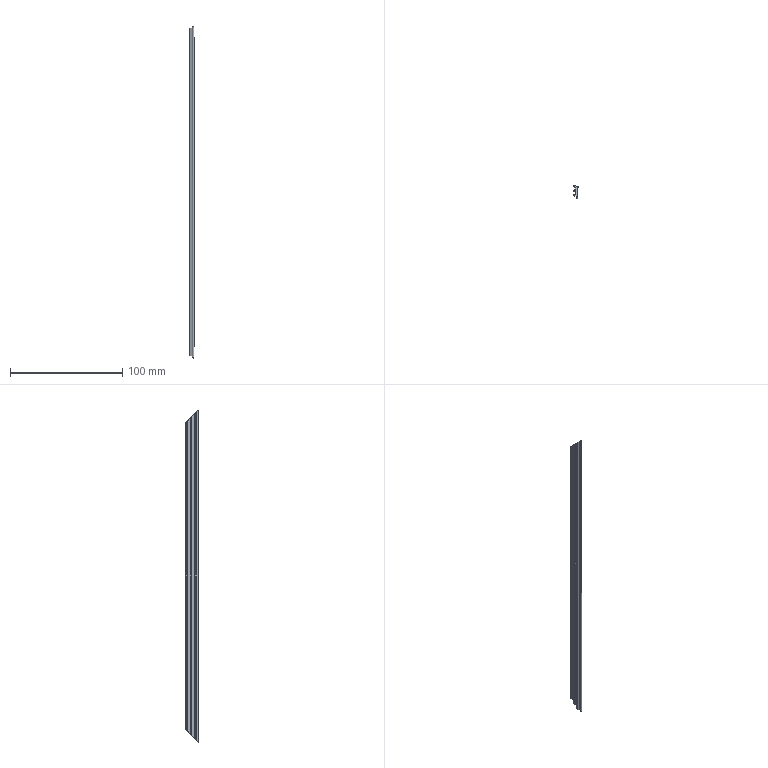Part | NX | features BREP 1 | 1 solid | 28 faces | box 3.587 x 11.224 x 296 mm | volume 6634 mm3 | plane 18 | cylinder 10 | commonest cylinder face diameters 0.4 x6 0.6 x2 1.942 x2
STEP:
#1=CARTESIAN_POINT('',(3.587,9.871,-138.128));
#2=VERTEX_POINT('',#1);
#3=CARTESIAN_POINT('',(3.287,9.567,-138.432));
#4=VERTEX_POINT('',#3);
#5=CARTESIAN_POINT('',(3.587,9.871,-138.128));
#6=CARTESIAN_POINT('',(3.589,9.693,-138.306));
#7=CARTESIAN_POINT('',(3.464,9.567,-138.432));
#8=CARTESIAN_POINT('',(3.287,9.567,-138.432));
#9=(BOUNDED_CURVE()B_SPLINE_CURVE(3,(#5,#6,#7,#8),.UNSPECIFIED.,.F.,.F.)B_SPLINE_CURVE_WITH_KNOTS((4,4),(4.699,6.283),.UNSPECIFIED.)CURVE()GEOMETRIC_REPRESENTATION_ITEM()RATIONAL_B_SPLINE_CURVE((1.,0.8015,0.8015,1.))REPRESENTATION_ITEM(''));
#10=EDGE_CURVE('',#2,#4,#9,.T.);
#11=ORIENTED_EDGE('',*,*,#10,.F.);
#12=CARTESIAN_POINT('',(3.587,9.871,138.128));
#13=VERTEX_POINT('',#12);
#14=CARTESIAN_POINT('',(3.587,9.871,148.));
#15=DIRECTION('',(0.,0.,-1.));
#16=VECTOR('',#15,1000.);
#17=LINE('',#14,#16);
#18=EDGE_CURVE('',#13,#2,#17,.T.);
#19=ORIENTED_EDGE('',*,*,#18,.F.);
#20=CARTESIAN_POINT('',(3.287,9.567,138.432));
#21=VERTEX_POINT('',#20);
#22=CARTESIAN_POINT('',(3.287,9.567,138.432));
#23=CARTESIAN_POINT('',(3.464,9.567,138.432));
#24=CARTESIAN_POINT('',(3.589,9.693,138.306));
#25=CARTESIAN_POINT('',(3.587,9.871,138.128));
#26=(BOUNDED_CURVE()B_SPLINE_CURVE(3,(#22,#23,#24,#25),.UNSPECIFIED.,.F.,.F.)B_SPLINE_CURVE_WITH_KNOTS((4,4),(3.142,4.726),.UNSPECIFIED.)CURVE()GEOMETRIC_REPRESENTATION_ITEM()RATIONAL_B_SPLINE_CURVE((1.,0.8015,0.8015,1.))REPRESENTATION_ITEM(''));
#27=EDGE_CURVE('',#21,#13,#26,.T.);
#28=ORIENTED_EDGE('',*,*,#27,.F.);
#29=CARTESIAN_POINT('',(3.287,9.567,148.));
#30=DIRECTION('',(0.,0.,-1.));
#31=VECTOR('',#30,1000.);
#32=LINE('',#29,#31);
#33=EDGE_CURVE('',#21,#4,#32,.T.);
#34=ORIENTED_EDGE('',*,*,#33,.T.);
#35=EDGE_LOOP('',(#11,#19,#28,#34));
#36=FACE_BOUND('',#35,.T.);
#37=CARTESIAN_POINT('',(3.287,9.867,148.));
#38=DIRECTION('',(0.,0.,-1.));
#39=DIRECTION('',(-1.,0.,0.));
#40=AXIS2_PLACEMENT_3D('',#37,#38,#39);
#41=CYLINDRICAL_SURFACE('',#40,0.3);
#42=ADVANCED_FACE('',(#36),#41,.T.);
#43=CARTESIAN_POINT('',(3.447,10.36,-137.639));
#44=VERTEX_POINT('',#43);
#45=CARTESIAN_POINT('',(3.447,10.36,-137.639));
#46=CARTESIAN_POINT('',(3.536,10.211,-137.788));
#47=CARTESIAN_POINT('',(3.584,10.044,-137.955));
#48=CARTESIAN_POINT('',(3.587,9.871,-138.128));
#49=(BOUNDED_CURVE()B_SPLINE_CURVE(3,(#45,#46,#47,#48),.UNSPECIFIED.,.F.,.F.)B_SPLINE_CURVE_WITH_KNOTS((4,4),(4.169,4.699),.UNSPECIFIED.)CURVE()GEOMETRIC_REPRESENTATION_ITEM()RATIONAL_B_SPLINE_CURVE((1.,0.9767,0.9767,1.))REPRESENTATION_ITEM(''));
#50=EDGE_CURVE('',#44,#2,#49,.T.);
#51=ORIENTED_EDGE('',*,*,#50,.F.);
#52=CARTESIAN_POINT('',(3.447,10.36,137.639));
#53=VERTEX_POINT('',#52);
#54=CARTESIAN_POINT('',(3.447,10.36,148.));
#55=DIRECTION('',(0.,0.,-1.));
#56=VECTOR('',#55,1000.);
#57=LINE('',#54,#56);
#58=EDGE_CURVE('',#53,#44,#57,.T.);
#59=ORIENTED_EDGE('',*,*,#58,.F.);
#60=CARTESIAN_POINT('',(3.587,9.871,138.128));
#61=CARTESIAN_POINT('',(3.584,10.044,137.955));
#62=CARTESIAN_POINT('',(3.536,10.211,137.788));
#63=CARTESIAN_POINT('',(3.447,10.36,137.639));
#64=(BOUNDED_CURVE()B_SPLINE_CURVE(3,(#60,#61,#62,#63),.UNSPECIFIED.,.F.,.F.)B_SPLINE_CURVE_WITH_KNOTS((4,4),(4.726,5.256),.UNSPECIFIED.)CURVE()GEOMETRIC_REPRESENTATION_ITEM()RATIONAL_B_SPLINE_CURVE((1.,0.9767,0.9767,1.))REPRESENTATION_ITEM(''));
#65=EDGE_CURVE('',#13,#53,#64,.T.);
#66=ORIENTED_EDGE('',*,*,#65,.F.);
#67=ORIENTED_EDGE('',*,*,#18,.T.);
#68=EDGE_LOOP('',(#51,#59,#66,#67));
#69=FACE_BOUND('',#68,.T.);
#70=CARTESIAN_POINT('',(2.616,9.857,148.));
#71=DIRECTION('',(0.,0.,-1.));
#72=DIRECTION('',(-1.,0.,0.));
#73=AXIS2_PLACEMENT_3D('',#70,#71,#72);
#74=CYLINDRICAL_SURFACE('',#73,0.971);
#75=ADVANCED_FACE('',(#69),#74,.T.);
#76=CARTESIAN_POINT('',(0.2517,11.216,-136.783));
#77=VERTEX_POINT('',#76);
#78=CARTESIAN_POINT('',(-63.462,28.281,-119.717));
#79=DIRECTION('',(0.9352,-0.2505,-0.2505));
#80=VECTOR('',#79,1000.);
#81=LINE('',#78,#80);
#82=EDGE_CURVE('',#77,#44,#81,.T.);
#83=ORIENTED_EDGE('',*,*,#82,.F.);
#84=CARTESIAN_POINT('',(0.2517,11.216,136.783));
#85=VERTEX_POINT('',#84);
#86=CARTESIAN_POINT('',(0.2517,11.216,148.));
#87=DIRECTION('',(0.,0.,-1.));
#88=VECTOR('',#87,1000.);
#89=LINE('',#86,#88);
#90=EDGE_CURVE('',#85,#77,#89,.T.);
#91=ORIENTED_EDGE('',*,*,#90,.F.);
#92=CARTESIAN_POINT('',(5.874,9.71,138.289));
#93=DIRECTION('',(-0.9352,0.2505,-0.2505));
#94=VECTOR('',#93,1000.);
#95=LINE('',#92,#94);
#96=EDGE_CURVE('',#53,#85,#95,.T.);
#97=ORIENTED_EDGE('',*,*,#96,.F.);
#98=ORIENTED_EDGE('',*,*,#58,.T.);
#99=EDGE_LOOP('',(#83,#91,#97,#98));
#100=FACE_BOUND('',#99,.T.);
#101=CARTESIAN_POINT('',(3.447,10.36,148.));
#102=DIRECTION('',(-0.2587,-0.9659,0.));
#103=DIRECTION('',(-0.9659,0.2587,0.));
#104=AXIS2_PLACEMENT_3D('',#101,#102,#103);
#105=PLANE('',#104);
#106=ADVANCED_FACE('',(#100),#105,.F.);
#107=CARTESIAN_POINT('',(0.,11.022,-136.976));
#108=VERTEX_POINT('',#107);
#109=CARTESIAN_POINT('',(0.,11.022,-136.976));
#110=CARTESIAN_POINT('',(0.,11.165,-136.833));
#111=CARTESIAN_POINT('',(0.1135,11.253,-136.746));
#112=CARTESIAN_POINT('',(0.2517,11.216,-136.783));
#113=(BOUNDED_CURVE()B_SPLINE_CURVE(3,(#109,#110,#111,#112),.UNSPECIFIED.,.F.,.F.)B_SPLINE_CURVE_WITH_KNOTS((4,4),(1.571,3.403),.UNSPECIFIED.)CURVE()GEOMETRIC_REPRESENTATION_ITEM()RATIONAL_B_SPLINE_CURVE((1.,0.7392,0.7392,1.))REPRESENTATION_ITEM(''));
#114=EDGE_CURVE('',#108,#77,#113,.T.);
#115=ORIENTED_EDGE('',*,*,#114,.F.);
#116=CARTESIAN_POINT('',(0.,11.022,136.976));
#117=VERTEX_POINT('',#116);
#118=CARTESIAN_POINT('',(0.,11.022,148.));
#119=DIRECTION('',(0.,0.,-1.));
#120=VECTOR('',#119,1000.);
#121=LINE('',#118,#120);
#122=EDGE_CURVE('',#117,#108,#121,.T.);
#123=ORIENTED_EDGE('',*,*,#122,.F.);
#124=CARTESIAN_POINT('',(0.2517,11.216,136.783));
#125=CARTESIAN_POINT('',(0.1135,11.253,136.746));
#126=CARTESIAN_POINT('',(0.,11.165,136.833));
#127=CARTESIAN_POINT('',(0.,11.022,136.976));
#128=(BOUNDED_CURVE()B_SPLINE_CURVE(3,(#124,#125,#126,#127),.UNSPECIFIED.,.F.,.F.)B_SPLINE_CURVE_WITH_KNOTS((4,4),(6.021,7.854),.UNSPECIFIED.)CURVE()GEOMETRIC_REPRESENTATION_ITEM()RATIONAL_B_SPLINE_CURVE((1.,0.7392,0.7392,1.))REPRESENTATION_ITEM(''));
#129=EDGE_CURVE('',#85,#117,#128,.T.);
#130=ORIENTED_EDGE('',*,*,#129,.F.);
#131=ORIENTED_EDGE('',*,*,#90,.T.);
#132=EDGE_LOOP('',(#115,#123,#130,#131));
#133=FACE_BOUND('',#132,.T.);
#134=CARTESIAN_POINT('',(0.2,11.022,148.));
#135=DIRECTION('',(0.,0.,-1.));
#136=DIRECTION('',(-1.,0.,0.));
#137=AXIS2_PLACEMENT_3D('',#134,#135,#136);
#138=CYLINDRICAL_SURFACE('',#137,0.2);
#139=ADVANCED_FACE('',(#133),#138,.T.);
#140=CARTESIAN_POINT('',(0.,10.432,-137.567));
#141=VERTEX_POINT('',#140);
#142=CARTESIAN_POINT('',(0.,153.511,5.512));
#143=DIRECTION('',(0.,0.7071,0.7071));
#144=VECTOR('',#143,1000.);
#145=LINE('',#142,#144);
#146=EDGE_CURVE('',#141,#108,#145,.T.);
#147=ORIENTED_EDGE('',*,*,#146,.F.);
#148=CARTESIAN_POINT('',(0.,10.432,137.567));
#149=VERTEX_POINT('',#148);
#150=CARTESIAN_POINT('',(0.,10.432,148.));
#151=DIRECTION('',(0.,0.,-1.));
#152=VECTOR('',#151,1000.);
#153=LINE('',#150,#152);
#154=EDGE_CURVE('',#149,#141,#153,.T.);
#155=ORIENTED_EDGE('',*,*,#154,.F.);
#156=CARTESIAN_POINT('',(0.,5.511,142.488));
#157=DIRECTION('',(0.,-0.7071,0.7071));
#158=VECTOR('',#157,1000.);
#159=LINE('',#156,#158);
#160=EDGE_CURVE('',#117,#149,#159,.T.);
#161=ORIENTED_EDGE('',*,*,#160,.F.);
#162=ORIENTED_EDGE('',*,*,#122,.T.);
#163=EDGE_LOOP('',(#147,#155,#161,#162));
#164=FACE_BOUND('',#163,.T.);
#165=CARTESIAN_POINT('',(0.,11.022,148.));
#166=DIRECTION('',(1.,0.,0.));
#167=DIRECTION('',(0.,1.,0.));
#168=AXIS2_PLACEMENT_3D('',#165,#166,#167);
#169=PLANE('',#168);
#170=ADVANCED_FACE('',(#164),#169,.F.);
#171=CARTESIAN_POINT('',(0.1483,10.238,-137.76));
#172=VERTEX_POINT('',#171);
#173=CARTESIAN_POINT('',(0.1483,10.238,-137.76));
#174=CARTESIAN_POINT('',(0.05733,10.263,-137.736));
#175=CARTESIAN_POINT('',(0.,10.338,-137.661));
#176=CARTESIAN_POINT('',(0.,10.432,-137.567));
#177=(BOUNDED_CURVE()B_SPLINE_CURVE(3,(#173,#174,#175,#176),.UNSPECIFIED.,.F.,.F.)B_SPLINE_CURVE_WITH_KNOTS((4,4),(0.2616,1.571),.UNSPECIFIED.)CURVE()GEOMETRIC_REPRESENTATION_ITEM()RATIONAL_B_SPLINE_CURVE((1.,0.8622,0.8622,1.))REPRESENTATION_ITEM(''));
#178=EDGE_CURVE('',#172,#141,#177,.T.);
#179=ORIENTED_EDGE('',*,*,#178,.F.);
#180=CARTESIAN_POINT('',(0.1483,10.238,137.76));
#181=VERTEX_POINT('',#180);
#182=CARTESIAN_POINT('',(0.1483,10.238,148.));
#183=DIRECTION('',(0.,0.,-1.));
#184=VECTOR('',#183,1000.);
#185=LINE('',#182,#184);
#186=EDGE_CURVE('',#181,#172,#185,.T.);
#187=ORIENTED_EDGE('',*,*,#186,.F.);
#188=CARTESIAN_POINT('',(0.,10.432,137.567));
#189=CARTESIAN_POINT('',(0.,10.338,137.661));
#190=CARTESIAN_POINT('',(0.05733,10.263,137.736));
#191=CARTESIAN_POINT('',(0.1483,10.238,137.76));
#192=(BOUNDED_CURVE()B_SPLINE_CURVE(3,(#188,#189,#190,#191),.UNSPECIFIED.,.F.,.F.)B_SPLINE_CURVE_WITH_KNOTS((4,4),(1.571,2.88),.UNSPECIFIED.)CURVE()GEOMETRIC_REPRESENTATION_ITEM()RATIONAL_B_SPLINE_CURVE((1.,0.8622,0.8622,1.))REPRESENTATION_ITEM(''));
#193=EDGE_CURVE('',#149,#181,#192,.T.);
#194=ORIENTED_EDGE('',*,*,#193,.F.);
#195=ORIENTED_EDGE('',*,*,#154,.T.);
#196=EDGE_LOOP('',(#179,#187,#194,#195));
#197=FACE_BOUND('',#196,.T.);
#198=CARTESIAN_POINT('',(0.2,10.432,148.));
#199=DIRECTION('',(0.,0.,-1.));
#200=DIRECTION('',(-1.,0.,0.));
#201=AXIS2_PLACEMENT_3D('',#198,#199,#200);
#202=CYLINDRICAL_SURFACE('',#201,0.2);
#203=ADVANCED_FACE('',(#197),#202,.T.);
#204=CARTESIAN_POINT('',(0.854,10.05,-137.949));
#205=VERTEX_POINT('',#204);
#206=CARTESIAN_POINT('',(-66.763,28.152,-119.847));
#207=DIRECTION('',(-0.9352,0.2504,0.2504));
#208=VECTOR('',#207,1000.);
#209=LINE('',#206,#208);
#210=EDGE_CURVE('',#205,#172,#209,.T.);
#211=ORIENTED_EDGE('',*,*,#210,.F.);
#212=CARTESIAN_POINT('',(0.854,10.05,137.949));
#213=VERTEX_POINT('',#212);
#214=CARTESIAN_POINT('',(0.854,10.05,148.));
#215=DIRECTION('',(0.,0.,-1.));
#216=VECTOR('',#215,1000.);
#217=LINE('',#214,#216);
#218=EDGE_CURVE('',#213,#205,#217,.T.);
#219=ORIENTED_EDGE('',*,*,#218,.F.);
#220=CARTESIAN_POINT('',(2.546,9.597,138.402));
#221=DIRECTION('',(0.9352,-0.2504,0.2504));
#222=VECTOR('',#221,1000.);
#223=LINE('',#220,#222);
#224=EDGE_CURVE('',#181,#213,#223,.T.);
#225=ORIENTED_EDGE('',*,*,#224,.F.);
#226=ORIENTED_EDGE('',*,*,#186,.T.);
#227=EDGE_LOOP('',(#211,#219,#225,#226));
#228=FACE_BOUND('',#227,.T.);
#229=CARTESIAN_POINT('',(0.1483,10.238,148.));
#230=DIRECTION('',(0.2586,0.966,0.));
#231=DIRECTION('',(0.,0.,-1.));
#232=AXIS2_PLACEMENT_3D('',#229,#230,#231);
#233=PLANE('',#232);
#234=ADVANCED_FACE('',(#228),#233,.F.);
#235=CARTESIAN_POINT('',(1.256,6.926,-141.073));
#236=VERTEX_POINT('',#235);
#237=CARTESIAN_POINT('',(-17.383,151.851,3.853));
#238=DIRECTION('',(-0.09057,0.7042,0.7042));
#239=VECTOR('',#238,1000.);
#240=LINE('',#237,#239);
#241=EDGE_CURVE('',#236,#205,#240,.T.);
#242=ORIENTED_EDGE('',*,*,#241,.F.);
#243=CARTESIAN_POINT('',(1.256,6.926,141.073));
#244=VERTEX_POINT('',#243);
#245=CARTESIAN_POINT('',(1.256,6.926,148.));
#246=DIRECTION('',(0.,0.,-1.));
#247=VECTOR('',#246,1000.);
#248=LINE('',#245,#247);
#249=EDGE_CURVE('',#244,#236,#248,.T.);
#250=ORIENTED_EDGE('',*,*,#249,.F.);
#251=CARTESIAN_POINT('',(1.495,5.065,142.933));
#252=DIRECTION('',(0.09057,-0.7042,0.7042));
#253=VECTOR('',#252,1000.);
#254=LINE('',#251,#253);
#255=EDGE_CURVE('',#213,#244,#254,.T.);
#256=ORIENTED_EDGE('',*,*,#255,.F.);
#257=ORIENTED_EDGE('',*,*,#218,.T.);
#258=EDGE_LOOP('',(#242,#250,#256,#257));
#259=FACE_BOUND('',#258,.T.);
#260=CARTESIAN_POINT('',(0.854,10.05,148.));
#261=DIRECTION('',(0.9918,0.1276,0.));
#262=DIRECTION('',(0.,0.,-1.));
#263=AXIS2_PLACEMENT_3D('',#260,#261,#262);
#264=PLANE('',#263);
#265=ADVANCED_FACE('',(#259),#264,.F.);
#266=CARTESIAN_POINT('',(0.2517,7.195,-140.804));
#267=VERTEX_POINT('',#266);
#268=CARTESIAN_POINT('',(-66.433,25.048,-122.951));
#269=DIRECTION('',(0.9352,-0.2504,-0.2504));
#270=VECTOR('',#269,1000.);
#271=LINE('',#268,#270);
#272=EDGE_CURVE('',#267,#236,#271,.T.);
#273=ORIENTED_EDGE('',*,*,#272,.F.);
#274=CARTESIAN_POINT('',(0.2517,7.195,140.804));
#275=VERTEX_POINT('',#274);
#276=CARTESIAN_POINT('',(0.2517,7.195,148.));
#277=DIRECTION('',(0.,0.,-1.));
#278=VECTOR('',#277,1000.);
#279=LINE('',#276,#278);
#280=EDGE_CURVE('',#275,#267,#279,.T.);
#281=ORIENTED_EDGE('',*,*,#280,.F.);
#282=CARTESIAN_POINT('',(2.878,6.492,141.507));
#283=DIRECTION('',(-0.9352,0.2504,-0.2504));
#284=VECTOR('',#283,1000.);
#285=LINE('',#282,#284);
#286=EDGE_CURVE('',#244,#275,#285,.T.);
#287=ORIENTED_EDGE('',*,*,#286,.F.);
#288=ORIENTED_EDGE('',*,*,#249,.T.);
#289=EDGE_LOOP('',(#273,#281,#287,#288));
#290=FACE_BOUND('',#289,.T.);
#291=CARTESIAN_POINT('',(1.256,6.926,148.));
#292=DIRECTION('',(-0.2586,-0.966,0.));
#293=DIRECTION('',(-0.966,0.2586,0.));
#294=AXIS2_PLACEMENT_3D('',#291,#292,#293);
#295=PLANE('',#294);
#296=ADVANCED_FACE('',(#290),#295,.F.);
#297=CARTESIAN_POINT('',(0.,7.001,-140.997));
#298=VERTEX_POINT('',#297);
#299=CARTESIAN_POINT('',(0.,7.001,-140.997));
#300=CARTESIAN_POINT('',(0.,7.145,-140.854));
#301=CARTESIAN_POINT('',(0.1135,7.232,-140.767));
#302=CARTESIAN_POINT('',(0.2517,7.195,-140.804));
#303=(BOUNDED_CURVE()B_SPLINE_CURVE(3,(#299,#300,#301,#302),.UNSPECIFIED.,.F.,.F.)B_SPLINE_CURVE_WITH_KNOTS((4,4),(1.571,3.403),.UNSPECIFIED.)CURVE()GEOMETRIC_REPRESENTATION_ITEM()RATIONAL_B_SPLINE_CURVE((1.,0.7392,0.7392,1.))REPRESENTATION_ITEM(''));
#304=EDGE_CURVE('',#298,#267,#303,.T.);
#305=ORIENTED_EDGE('',*,*,#304,.F.);
#306=CARTESIAN_POINT('',(0.,7.001,140.997));
#307=VERTEX_POINT('',#306);
#308=CARTESIAN_POINT('',(0.,7.001,148.));
#309=DIRECTION('',(0.,0.,-1.));
#310=VECTOR('',#309,1000.);
#311=LINE('',#308,#310);
#312=EDGE_CURVE('',#307,#298,#311,.T.);
#313=ORIENTED_EDGE('',*,*,#312,.F.);
#314=CARTESIAN_POINT('',(0.2517,7.195,140.804));
#315=CARTESIAN_POINT('',(0.1135,7.232,140.767));
#316=CARTESIAN_POINT('',(0.,7.145,140.854));
#317=CARTESIAN_POINT('',(0.,7.001,140.997));
#318=(BOUNDED_CURVE()B_SPLINE_CURVE(3,(#314,#315,#316,#317),.UNSPECIFIED.,.F.,.F.)B_SPLINE_CURVE_WITH_KNOTS((4,4),(6.022,7.854),.UNSPECIFIED.)CURVE()GEOMETRIC_REPRESENTATION_ITEM()RATIONAL_B_SPLINE_CURVE((1.,0.7392,0.7392,1.))REPRESENTATION_ITEM(''));
#319=EDGE_CURVE('',#275,#307,#318,.T.);
#320=ORIENTED_EDGE('',*,*,#319,.F.);
#321=ORIENTED_EDGE('',*,*,#280,.T.);
#322=EDGE_LOOP('',(#305,#313,#320,#321));
#323=FACE_BOUND('',#322,.T.);
#324=CARTESIAN_POINT('',(0.2,7.001,148.));
#325=DIRECTION('',(0.,0.,-1.));
#326=DIRECTION('',(-1.,0.,0.));
#327=AXIS2_PLACEMENT_3D('',#324,#325,#326);
#328=CYLINDRICAL_SURFACE('',#327,0.2);
#329=ADVANCED_FACE('',(#323),#328,.T.);
#330=CARTESIAN_POINT('',(0.,6.41,-141.589));
#331=VERTEX_POINT('',#330);
#332=CARTESIAN_POINT('',(0.,151.5,3.501));
#333=DIRECTION('',(0.,0.7071,0.7071));
#334=VECTOR('',#333,1000.);
#335=LINE('',#332,#334);
#336=EDGE_CURVE('',#331,#298,#335,.T.);
#337=ORIENTED_EDGE('',*,*,#336,.F.);
#338=CARTESIAN_POINT('',(0.,6.41,141.589));
#339=VERTEX_POINT('',#338);
#340=CARTESIAN_POINT('',(0.,6.41,148.));
#341=DIRECTION('',(0.,0.,-1.));
#342=VECTOR('',#341,1000.);
#343=LINE('',#340,#342);
#344=EDGE_CURVE('',#339,#331,#343,.T.);
#345=ORIENTED_EDGE('',*,*,#344,.F.);
#346=CARTESIAN_POINT('',(0.,3.5,144.499));
#347=DIRECTION('',(0.,-0.7071,0.7071));
#348=VECTOR('',#347,1000.);
#349=LINE('',#346,#348);
#350=EDGE_CURVE('',#307,#339,#349,.T.);
#351=ORIENTED_EDGE('',*,*,#350,.F.);
#352=ORIENTED_EDGE('',*,*,#312,.T.);
#353=EDGE_LOOP('',(#337,#345,#351,#352));
#354=FACE_BOUND('',#353,.T.);
#355=CARTESIAN_POINT('',(0.,7.001,148.));
#356=DIRECTION('',(1.,0.,0.));
#357=DIRECTION('',(0.,1.,0.));
#358=AXIS2_PLACEMENT_3D('',#355,#356,#357);
#359=PLANE('',#358);
#360=ADVANCED_FACE('',(#354),#359,.F.);
#361=CARTESIAN_POINT('',(0.1482,6.217,-141.782));
#362=VERTEX_POINT('',#361);
#363=CARTESIAN_POINT('',(0.1482,6.217,-141.782));
#364=CARTESIAN_POINT('',(0.0573,6.241,-141.758));
#365=CARTESIAN_POINT('',(0.,6.316,-141.683));
#366=CARTESIAN_POINT('',(0.,6.41,-141.589));
#367=(BOUNDED_CURVE()B_SPLINE_CURVE(3,(#363,#364,#365,#366),.UNSPECIFIED.,.F.,.F.)B_SPLINE_CURVE_WITH_KNOTS((4,4),(0.2619,1.571),.UNSPECIFIED.)CURVE()GEOMETRIC_REPRESENTATION_ITEM()RATIONAL_B_SPLINE_CURVE((1.,0.8623,0.8623,1.))REPRESENTATION_ITEM(''));
#368=EDGE_CURVE('',#362,#331,#367,.T.);
#369=ORIENTED_EDGE('',*,*,#368,.F.);
#370=CARTESIAN_POINT('',(0.1482,6.217,141.782));
#371=VERTEX_POINT('',#370);
#372=CARTESIAN_POINT('',(0.1482,6.217,148.));
#373=DIRECTION('',(0.,0.,-1.));
#374=VECTOR('',#373,1000.);
#375=LINE('',#372,#374);
#376=EDGE_CURVE('',#371,#362,#375,.T.);
#377=ORIENTED_EDGE('',*,*,#376,.F.);
#378=CARTESIAN_POINT('',(0.,6.41,141.589));
#379=CARTESIAN_POINT('',(0.,6.316,141.683));
#380=CARTESIAN_POINT('',(0.0573,6.241,141.758));
#381=CARTESIAN_POINT('',(0.1482,6.217,141.782));
#382=(BOUNDED_CURVE()B_SPLINE_CURVE(3,(#378,#379,#380,#381),.UNSPECIFIED.,.F.,.F.)B_SPLINE_CURVE_WITH_KNOTS((4,4),(1.571,2.88),.UNSPECIFIED.)CURVE()GEOMETRIC_REPRESENTATION_ITEM()RATIONAL_B_SPLINE_CURVE((1.,0.8623,0.8623,1.))REPRESENTATION_ITEM(''));
#383=EDGE_CURVE('',#339,#371,#382,.T.);
#384=ORIENTED_EDGE('',*,*,#383,.F.);
#385=ORIENTED_EDGE('',*,*,#344,.T.);
#386=EDGE_LOOP('',(#369,#377,#384,#385));
#387=FACE_BOUND('',#386,.T.);
#388=CARTESIAN_POINT('',(0.2,6.41,148.));
#389=DIRECTION('',(0.,0.,-1.));
#390=DIRECTION('',(-1.,0.,0.));
#391=AXIS2_PLACEMENT_3D('',#388,#389,#390);
#392=CYLINDRICAL_SURFACE('',#391,0.2);
#393=ADVANCED_FACE('',(#387),#392,.T.);
#394=CARTESIAN_POINT('',(1.39,5.884,-142.115));
#395=VERTEX_POINT('',#394);
#396=CARTESIAN_POINT('',(-67.774,24.426,-123.573));
#397=DIRECTION('',(-0.9351,0.2507,0.2507));
#398=VECTOR('',#397,1000.);
#399=LINE('',#396,#398);
#400=EDGE_CURVE('',#395,#362,#399,.T.);
#401=ORIENTED_EDGE('',*,*,#400,.F.);
#402=CARTESIAN_POINT('',(1.39,5.884,142.115));
#403=VERTEX_POINT('',#402);
#404=CARTESIAN_POINT('',(1.39,5.884,148.));
#405=DIRECTION('',(0.,0.,-1.));
#406=VECTOR('',#405,1000.);
#407=LINE('',#404,#406);
#408=EDGE_CURVE('',#403,#395,#407,.T.);
#409=ORIENTED_EDGE('',*,*,#408,.F.);
#410=CARTESIAN_POINT('',(1.606,5.826,142.173));
#411=DIRECTION('',(0.9351,-0.2507,0.2507));
#412=VECTOR('',#411,1000.);
#413=LINE('',#410,#412);
#414=EDGE_CURVE('',#371,#403,#413,.T.);
#415=ORIENTED_EDGE('',*,*,#414,.F.);
#416=ORIENTED_EDGE('',*,*,#376,.T.);
#417=EDGE_LOOP('',(#401,#409,#415,#416));
#418=FACE_BOUND('',#417,.T.);
#419=CARTESIAN_POINT('',(0.1482,6.217,148.));
#420=DIRECTION('',(0.2589,0.9659,0.));
#421=DIRECTION('',(0.,0.,-1.));
#422=AXIS2_PLACEMENT_3D('',#419,#420,#421);
#423=PLANE('',#422);
#424=ADVANCED_FACE('',(#418),#423,.F.);
#425=CARTESIAN_POINT('',(1.791,2.761,-145.238));
#426=VERTEX_POINT('',#425);
#427=CARTESIAN_POINT('',(-17.113,149.751,1.753));
#428=DIRECTION('',(-0.09057,0.7042,0.7042));
#429=VECTOR('',#428,1000.);
#430=LINE('',#427,#429);
#431=EDGE_CURVE('',#426,#395,#430,.T.);
#432=ORIENTED_EDGE('',*,*,#431,.F.);
#433=CARTESIAN_POINT('',(1.791,2.761,145.238));
#434=VERTEX_POINT('',#433);
#435=CARTESIAN_POINT('',(1.791,2.761,148.));
#436=DIRECTION('',(0.,0.,-1.));
#437=VECTOR('',#436,1000.);
#438=LINE('',#435,#437);
#439=EDGE_CURVE('',#434,#426,#438,.T.);
#440=ORIENTED_EDGE('',*,*,#439,.F.);
#441=CARTESIAN_POINT('',(1.765,2.965,145.033));
#442=DIRECTION('',(0.09057,-0.7042,0.7042));
#443=VECTOR('',#442,1000.);
#444=LINE('',#441,#443);
#445=EDGE_CURVE('',#403,#434,#444,.T.);
#446=ORIENTED_EDGE('',*,*,#445,.F.);
#447=ORIENTED_EDGE('',*,*,#408,.T.);
#448=EDGE_LOOP('',(#432,#440,#446,#447));
#449=FACE_BOUND('',#448,.T.);
#450=CARTESIAN_POINT('',(1.39,5.884,148.));
#451=DIRECTION('',(0.9918,0.1276,0.));
#452=DIRECTION('',(0.,0.,-1.));
#453=AXIS2_PLACEMENT_3D('',#450,#451,#452);
#454=PLANE('',#453);
#455=ADVANCED_FACE('',(#449),#454,.F.);
#456=CARTESIAN_POINT('',(0.2518,3.174,-144.825));
#457=VERTEX_POINT('',#456);
#458=CARTESIAN_POINT('',(-66.936,21.184,-126.815));
#459=DIRECTION('',(0.9351,-0.2506,-0.2506));
#460=VECTOR('',#459,1000.);
#461=LINE('',#458,#460);
#462=EDGE_CURVE('',#457,#426,#461,.T.);
#463=ORIENTED_EDGE('',*,*,#462,.F.);
#464=CARTESIAN_POINT('',(0.2518,3.174,144.825));
#465=VERTEX_POINT('',#464);
#466=CARTESIAN_POINT('',(0.2518,3.174,148.));
#467=DIRECTION('',(0.,0.,-1.));
#468=VECTOR('',#467,1000.);
#469=LINE('',#466,#468);
#470=EDGE_CURVE('',#465,#457,#469,.T.);
#471=ORIENTED_EDGE('',*,*,#470,.F.);
#472=CARTESIAN_POINT('',(2.439,2.588,145.411));
#473=DIRECTION('',(-0.9351,0.2506,-0.2506));
#474=VECTOR('',#473,1000.);
#475=LINE('',#472,#474);
#476=EDGE_CURVE('',#434,#465,#475,.T.);
#477=ORIENTED_EDGE('',*,*,#476,.F.);
#478=ORIENTED_EDGE('',*,*,#439,.T.);
#479=EDGE_LOOP('',(#463,#471,#477,#478));
#480=FACE_BOUND('',#479,.T.);
#481=CARTESIAN_POINT('',(1.791,2.761,148.));
#482=DIRECTION('',(-0.2589,-0.9659,0.));
#483=DIRECTION('',(-0.9659,0.2589,0.));
#484=AXIS2_PLACEMENT_3D('',#481,#482,#483);
#485=PLANE('',#484);
#486=ADVANCED_FACE('',(#480),#485,.F.);
#487=CARTESIAN_POINT('',(0.,2.981,-145.018));
#488=VERTEX_POINT('',#487);
#489=CARTESIAN_POINT('',(0.,2.981,-145.018));
#490=CARTESIAN_POINT('',(0.,3.124,-144.875));
#491=CARTESIAN_POINT('',(0.1135,3.211,-144.788));
#492=CARTESIAN_POINT('',(0.2518,3.174,-144.825));
#493=(BOUNDED_CURVE()B_SPLINE_CURVE(3,(#489,#490,#491,#492),.UNSPECIFIED.,.F.,.F.)B_SPLINE_CURVE_WITH_KNOTS((4,4),(1.571,3.403),.UNSPECIFIED.)CURVE()GEOMETRIC_REPRESENTATION_ITEM()RATIONAL_B_SPLINE_CURVE((1.,0.7391,0.7391,1.))REPRESENTATION_ITEM(''));
#494=EDGE_CURVE('',#488,#457,#493,.T.);
#495=ORIENTED_EDGE('',*,*,#494,.F.);
#496=CARTESIAN_POINT('',(0.,2.981,145.018));
#497=VERTEX_POINT('',#496);
#498=CARTESIAN_POINT('',(0.,2.981,148.));
#499=DIRECTION('',(0.,0.,-1.));
#500=VECTOR('',#499,1000.);
#501=LINE('',#498,#500);
#502=EDGE_CURVE('',#497,#488,#501,.T.);
#503=ORIENTED_EDGE('',*,*,#502,.F.);
#504=CARTESIAN_POINT('',(0.2518,3.174,144.825));
#505=CARTESIAN_POINT('',(0.1135,3.211,144.788));
#506=CARTESIAN_POINT('',(0.,3.124,144.875));
#507=CARTESIAN_POINT('',(0.,2.981,145.018));
#508=(BOUNDED_CURVE()B_SPLINE_CURVE(3,(#504,#505,#506,#507),.UNSPECIFIED.,.F.,.F.)B_SPLINE_CURVE_WITH_KNOTS((4,4),(6.021,7.854),.UNSPECIFIED.)CURVE()GEOMETRIC_REPRESENTATION_ITEM()RATIONAL_B_SPLINE_CURVE((1.,0.7391,0.7391,1.))REPRESENTATION_ITEM(''));
#509=EDGE_CURVE('',#465,#497,#508,.T.);
#510=ORIENTED_EDGE('',*,*,#509,.F.);
#511=ORIENTED_EDGE('',*,*,#470,.T.);
#512=EDGE_LOOP('',(#495,#503,#510,#511));
#513=FACE_BOUND('',#512,.T.);
#514=CARTESIAN_POINT('',(0.2,2.981,148.));
#515=DIRECTION('',(0.,0.,-1.));
#516=DIRECTION('',(-1.,0.,0.));
#517=AXIS2_PLACEMENT_3D('',#514,#515,#516);
#518=CYLINDRICAL_SURFACE('',#517,0.2);
#519=ADVANCED_FACE('',(#513),#518,.T.);
#520=CARTESIAN_POINT('',(0.,2.39,-145.609));
#521=VERTEX_POINT('',#520);
#522=CARTESIAN_POINT('',(0.,149.49,1.491));
#523=DIRECTION('',(0.,0.7071,0.7071));
#524=VECTOR('',#523,1000.);
#525=LINE('',#522,#524);
#526=EDGE_CURVE('',#521,#488,#525,.T.);
#527=ORIENTED_EDGE('',*,*,#526,.F.);
#528=CARTESIAN_POINT('',(0.,2.39,145.609));
#529=VERTEX_POINT('',#528);
#530=CARTESIAN_POINT('',(0.,2.39,148.));
#531=DIRECTION('',(0.,0.,-1.));
#532=VECTOR('',#531,1000.);
#533=LINE('',#530,#532);
#534=EDGE_CURVE('',#529,#521,#533,.T.);
#535=ORIENTED_EDGE('',*,*,#534,.F.);
#536=CARTESIAN_POINT('',(0.,1.49,146.509));
#537=DIRECTION('',(0.,-0.7071,0.7071));
#538=VECTOR('',#537,1000.);
#539=LINE('',#536,#538);
#540=EDGE_CURVE('',#497,#529,#539,.T.);
#541=ORIENTED_EDGE('',*,*,#540,.F.);
#542=ORIENTED_EDGE('',*,*,#502,.T.);
#543=EDGE_LOOP('',(#527,#535,#541,#542));
#544=FACE_BOUND('',#543,.T.);
#545=CARTESIAN_POINT('',(0.,2.981,148.));
#546=DIRECTION('',(1.,0.,0.));
#547=DIRECTION('',(0.,1.,0.));
#548=AXIS2_PLACEMENT_3D('',#545,#546,#547);
#549=PLANE('',#548);
#550=ADVANCED_FACE('',(#544),#549,.F.);
#551=CARTESIAN_POINT('',(0.1482,2.196,-145.802));
#552=VERTEX_POINT('',#551);
#553=CARTESIAN_POINT('',(0.1482,2.196,-145.802));
#554=CARTESIAN_POINT('',(0.05729,2.221,-145.778));
#555=CARTESIAN_POINT('',(0.,2.295,-145.703));
#556=CARTESIAN_POINT('',(0.,2.39,-145.609));
#557=(BOUNDED_CURVE()B_SPLINE_CURVE(3,(#553,#554,#555,#556),.UNSPECIFIED.,.F.,.F.)B_SPLINE_CURVE_WITH_KNOTS((4,4),(0.262,1.571),.UNSPECIFIED.)CURVE()GEOMETRIC_REPRESENTATION_ITEM()RATIONAL_B_SPLINE_CURVE((1.,0.8623,0.8623,1.))REPRESENTATION_ITEM(''));
#558=EDGE_CURVE('',#552,#521,#557,.T.);
#559=ORIENTED_EDGE('',*,*,#558,.F.);
#560=CARTESIAN_POINT('',(0.1482,2.196,145.802));
#561=VERTEX_POINT('',#560);
#562=CARTESIAN_POINT('',(0.1482,2.196,148.));
#563=DIRECTION('',(0.,0.,-1.));
#564=VECTOR('',#563,1000.);
#565=LINE('',#562,#564);
#566=EDGE_CURVE('',#561,#552,#565,.T.);
#567=ORIENTED_EDGE('',*,*,#566,.F.);
#568=CARTESIAN_POINT('',(0.,2.39,145.609));
#569=CARTESIAN_POINT('',(0.,2.295,145.703));
#570=CARTESIAN_POINT('',(0.05729,2.221,145.778));
#571=CARTESIAN_POINT('',(0.1482,2.196,145.802));
#572=(BOUNDED_CURVE()B_SPLINE_CURVE(3,(#568,#569,#570,#571),.UNSPECIFIED.,.F.,.F.)B_SPLINE_CURVE_WITH_KNOTS((4,4),(1.571,2.88),.UNSPECIFIED.)CURVE()GEOMETRIC_REPRESENTATION_ITEM()RATIONAL_B_SPLINE_CURVE((1.,0.8623,0.8623,1.))REPRESENTATION_ITEM(''));
#573=EDGE_CURVE('',#529,#561,#572,.T.);
#574=ORIENTED_EDGE('',*,*,#573,.F.);
#575=ORIENTED_EDGE('',*,*,#534,.T.);
#576=EDGE_LOOP('',(#559,#567,#574,#575));
#577=FACE_BOUND('',#576,.T.);
#578=CARTESIAN_POINT('',(0.2,2.39,148.));
#579=DIRECTION('',(0.,0.,-1.));
#580=DIRECTION('',(-1.,0.,0.));
#581=AXIS2_PLACEMENT_3D('',#578,#579,#580);
#582=CYLINDRICAL_SURFACE('',#581,0.2);
#583=ADVANCED_FACE('',(#577),#582,.T.);
#584=CARTESIAN_POINT('',(1.925,1.72,-146.279));
#585=VERTEX_POINT('',#584);
#586=CARTESIAN_POINT('',(-68.724,20.662,-127.337));
#587=DIRECTION('',(-0.935,0.2507,0.2507));
#588=VECTOR('',#587,1000.);
#589=LINE('',#586,#588);
#590=EDGE_CURVE('',#585,#552,#589,.T.);
#591=ORIENTED_EDGE('',*,*,#590,.F.);
#592=CARTESIAN_POINT('',(1.925,1.72,146.279));
#593=VERTEX_POINT('',#592);
#594=CARTESIAN_POINT('',(1.925,1.72,148.));
#595=DIRECTION('',(0.,0.,-1.));
#596=VECTOR('',#595,1000.);
#597=LINE('',#594,#596);
#598=EDGE_CURVE('',#593,#585,#597,.T.);
#599=ORIENTED_EDGE('',*,*,#598,.F.);
#600=CARTESIAN_POINT('',(0.6633,2.058,145.941));
#601=DIRECTION('',(0.935,-0.2507,0.2507));
#602=VECTOR('',#601,1000.);
#603=LINE('',#600,#602);
#604=EDGE_CURVE('',#561,#593,#603,.T.);
#605=ORIENTED_EDGE('',*,*,#604,.F.);
#606=ORIENTED_EDGE('',*,*,#566,.T.);
#607=EDGE_LOOP('',(#591,#599,#605,#606));
#608=FACE_BOUND('',#607,.T.);
#609=CARTESIAN_POINT('',(0.1482,2.196,148.));
#610=DIRECTION('',(0.259,0.9659,0.));
#611=DIRECTION('',(0.,0.,-1.));
#612=AXIS2_PLACEMENT_3D('',#609,#610,#611);
#613=PLANE('',#612);
#614=ADVANCED_FACE('',(#608),#613,.F.);
#615=CARTESIAN_POINT('',(2.108,0.3017,-147.697));
#616=VERTEX_POINT('',#615);
#617=CARTESIAN_POINT('',(-16.843,147.652,-0.3464));
#618=DIRECTION('',(-0.09057,0.7042,0.7042));
#619=VECTOR('',#618,1000.);
#620=LINE('',#617,#619);
#621=EDGE_CURVE('',#616,#585,#620,.T.);
#622=ORIENTED_EDGE('',*,*,#621,.F.);
#623=CARTESIAN_POINT('',(2.108,0.3017,147.697));
#624=VERTEX_POINT('',#623);
#625=CARTESIAN_POINT('',(2.108,0.3017,148.));
#626=DIRECTION('',(0.,0.,-1.));
#627=VECTOR('',#626,1000.);
#628=LINE('',#625,#627);
#629=EDGE_CURVE('',#624,#616,#628,.T.);
#630=ORIENTED_EDGE('',*,*,#629,.F.);
#631=CARTESIAN_POINT('',(2.035,0.8664,147.132));
#632=DIRECTION('',(0.09057,-0.7042,0.7042));
#633=VECTOR('',#632,1000.);
#634=LINE('',#631,#633);
#635=EDGE_CURVE('',#593,#624,#634,.T.);
#636=ORIENTED_EDGE('',*,*,#635,.F.);
#637=ORIENTED_EDGE('',*,*,#598,.T.);
#638=EDGE_LOOP('',(#622,#630,#636,#637));
#639=FACE_BOUND('',#638,.T.);
#640=CARTESIAN_POINT('',(1.925,1.72,148.));
#641=DIRECTION('',(0.9918,0.1276,0.));
#642=DIRECTION('',(0.,0.,-1.));
#643=AXIS2_PLACEMENT_3D('',#640,#641,#642);
#644=PLANE('',#643);
#645=ADVANCED_FACE('',(#639),#644,.F.);
#646=ORIENTED_EDGE('',*,*,#629,.T.);
#647=CARTESIAN_POINT('',(3.447,0.2347,-147.764));
#648=VERTEX_POINT('',#647);
#649=CARTESIAN_POINT('',(3.447,0.2347,-147.764));
#650=CARTESIAN_POINT('',(3.032,-0.1233,-148.122));
#651=CARTESIAN_POINT('',(2.485,-0.0959,-148.095));
#652=CARTESIAN_POINT('',(2.108,0.3017,-147.697));
#653=(BOUNDED_CURVE()B_SPLINE_CURVE(3,(#649,#650,#651,#652),.UNSPECIFIED.,.F.,.F.)B_SPLINE_CURVE_WITH_KNOTS((4,4),(5.571,7.095),.UNSPECIFIED.)CURVE()GEOMETRIC_REPRESENTATION_ITEM()RATIONAL_B_SPLINE_CURVE((1.,0.8156,0.8156,1.))REPRESENTATION_ITEM(''));
#654=EDGE_CURVE('',#648,#616,#653,.T.);
#655=ORIENTED_EDGE('',*,*,#654,.F.);
#656=CARTESIAN_POINT('',(3.447,0.2347,147.764));
#657=VERTEX_POINT('',#656);
#658=CARTESIAN_POINT('',(3.447,0.2347,148.));
#659=DIRECTION('',(0.,0.,-1.));
#660=VECTOR('',#659,1000.);
#661=LINE('',#658,#660);
#662=EDGE_CURVE('',#657,#648,#661,.T.);
#663=ORIENTED_EDGE('',*,*,#662,.F.);
#664=CARTESIAN_POINT('',(2.108,0.3017,147.697));
#665=CARTESIAN_POINT('',(2.485,-0.0959,148.095));
#666=CARTESIAN_POINT('',(3.032,-0.1233,148.122));
#667=CARTESIAN_POINT('',(3.447,0.2347,147.764));
#668=(BOUNDED_CURVE()B_SPLINE_CURVE(3,(#664,#665,#666,#667),.UNSPECIFIED.,.F.,.F.)B_SPLINE_CURVE_WITH_KNOTS((4,4),(2.33,3.854),.UNSPECIFIED.)CURVE()GEOMETRIC_REPRESENTATION_ITEM()RATIONAL_B_SPLINE_CURVE((1.,0.8156,0.8156,1.))REPRESENTATION_ITEM(''));
#669=EDGE_CURVE('',#624,#657,#668,.T.);
#670=ORIENTED_EDGE('',*,*,#669,.F.);
#671=EDGE_LOOP('',(#646,#655,#663,#670));
#672=FACE_BOUND('',#671,.T.);
#673=CARTESIAN_POINT('',(2.812,0.9697,148.));
#674=DIRECTION('',(0.,0.,-1.));
#675=DIRECTION('',(-1.,0.,0.));
#676=AXIS2_PLACEMENT_3D('',#673,#674,#675);
#677=CYLINDRICAL_SURFACE('',#676,0.971);
#678=ADVANCED_FACE('',(#672),#677,.T.);
#679=CARTESIAN_POINT('',(3.447,5.067,-142.932));
#680=VERTEX_POINT('',#679);
#681=CARTESIAN_POINT('',(3.447,148.117,0.1179));
#682=DIRECTION('',(0.,-0.7071,-0.7071));
#683=VECTOR('',#682,1000.);
#684=LINE('',#681,#683);
#685=EDGE_CURVE('',#680,#648,#684,.T.);
#686=ORIENTED_EDGE('',*,*,#685,.F.);
#687=CARTESIAN_POINT('',(3.447,5.067,142.932));
#688=VERTEX_POINT('',#687);
#689=CARTESIAN_POINT('',(3.447,5.067,148.));
#690=DIRECTION('',(0.,0.,-1.));
#691=VECTOR('',#690,1000.);
#692=LINE('',#689,#691);
#693=EDGE_CURVE('',#688,#680,#692,.T.);
#694=ORIENTED_EDGE('',*,*,#693,.F.);
#695=CARTESIAN_POINT('',(3.447,0.1167,147.882));
#696=DIRECTION('',(0.,0.7071,-0.7071));
#697=VECTOR('',#696,1000.);
#698=LINE('',#695,#697);
#699=EDGE_CURVE('',#657,#688,#698,.T.);
#700=ORIENTED_EDGE('',*,*,#699,.F.);
#701=ORIENTED_EDGE('',*,*,#662,.T.);
#702=EDGE_LOOP('',(#686,#694,#700,#701));
#703=FACE_BOUND('',#702,.T.);
#704=CARTESIAN_POINT('',(3.447,0.2347,148.));
#705=DIRECTION('',(-1.,0.,0.));
#706=DIRECTION('',(0.,0.,1.));
#707=AXIS2_PLACEMENT_3D('',#704,#705,#706);
#708=PLANE('',#707);
#709=ADVANCED_FACE('',(#703),#708,.F.);
#710=CARTESIAN_POINT('',(3.147,5.367,-142.632));
#711=VERTEX_POINT('',#710);
#712=CARTESIAN_POINT('',(3.147,5.367,-142.632));
#713=CARTESIAN_POINT('',(3.322,5.367,-142.632));
#714=CARTESIAN_POINT('',(3.447,5.242,-142.756));
#715=CARTESIAN_POINT('',(3.447,5.067,-142.932));
#716=(BOUNDED_CURVE()B_SPLINE_CURVE(3,(#712,#713,#714,#715),.UNSPECIFIED.,.F.,.F.)B_SPLINE_CURVE_WITH_KNOTS((4,4),(3.142,4.712),.UNSPECIFIED.)CURVE()GEOMETRIC_REPRESENTATION_ITEM()RATIONAL_B_SPLINE_CURVE((1.,0.8047,0.8047,1.))REPRESENTATION_ITEM(''));
#717=EDGE_CURVE('',#711,#680,#716,.T.);
#718=ORIENTED_EDGE('',*,*,#717,.F.);
#719=CARTESIAN_POINT('',(3.147,5.367,142.632));
#720=VERTEX_POINT('',#719);
#721=CARTESIAN_POINT('',(3.147,5.367,148.));
#722=DIRECTION('',(0.,0.,-1.));
#723=VECTOR('',#722,1000.);
#724=LINE('',#721,#723);
#725=EDGE_CURVE('',#720,#711,#724,.T.);
#726=ORIENTED_EDGE('',*,*,#725,.F.);
#727=CARTESIAN_POINT('',(3.447,5.067,142.932));
#728=CARTESIAN_POINT('',(3.447,5.242,142.756));
#729=CARTESIAN_POINT('',(3.322,5.367,142.632));
#730=CARTESIAN_POINT('',(3.147,5.367,142.632));
#731=(BOUNDED_CURVE()B_SPLINE_CURVE(3,(#727,#728,#729,#730),.UNSPECIFIED.,.F.,.F.)B_SPLINE_CURVE_WITH_KNOTS((4,4),(4.712,6.283),.UNSPECIFIED.)CURVE()GEOMETRIC_REPRESENTATION_ITEM()RATIONAL_B_SPLINE_CURVE((1.,0.8047,0.8047,1.))REPRESENTATION_ITEM(''));
#732=EDGE_CURVE('',#688,#720,#731,.T.);
#733=ORIENTED_EDGE('',*,*,#732,.F.);
#734=ORIENTED_EDGE('',*,*,#693,.T.);
#735=EDGE_LOOP('',(#718,#726,#733,#734));
#736=FACE_BOUND('',#735,.T.);
#737=CARTESIAN_POINT('',(3.147,5.067,148.));
#738=DIRECTION('',(0.,0.,-1.));
#739=DIRECTION('',(-1.,0.,0.));
#740=AXIS2_PLACEMENT_3D('',#737,#738,#739);
#741=CYLINDRICAL_SURFACE('',#740,0.3);
#742=ADVANCED_FACE('',(#736),#741,.T.);
#743=CARTESIAN_POINT('',(3.,5.367,-142.632));
#744=VERTEX_POINT('',#743);
#745=CARTESIAN_POINT('',(3.147,5.367,-142.632));
#746=DIRECTION('',(1.,0.,0.));
#747=VECTOR('',#746,1000.);
#748=LINE('',#745,#747);
#749=EDGE_CURVE('',#744,#711,#748,.T.);
#750=ORIENTED_EDGE('',*,*,#749,.F.);
#751=CARTESIAN_POINT('',(3.,5.367,142.632));
#752=VERTEX_POINT('',#751);
#753=CARTESIAN_POINT('',(3.,5.367,148.));
#754=DIRECTION('',(0.,0.,-1.));
#755=VECTOR('',#754,1000.);
#756=LINE('',#753,#755);
#757=EDGE_CURVE('',#752,#744,#756,.T.);
#758=ORIENTED_EDGE('',*,*,#757,.F.);
#759=CARTESIAN_POINT('',(3.147,5.367,142.632));
#760=DIRECTION('',(-1.,0.,0.));
#761=VECTOR('',#760,1000.);
#762=LINE('',#759,#761);
#763=EDGE_CURVE('',#720,#752,#762,.T.);
#764=ORIENTED_EDGE('',*,*,#763,.F.);
#765=ORIENTED_EDGE('',*,*,#725,.T.);
#766=EDGE_LOOP('',(#750,#758,#764,#765));
#767=FACE_BOUND('',#766,.T.);
#768=CARTESIAN_POINT('',(3.147,5.367,148.));
#769=DIRECTION('',(0.,-1.,0.));
#770=DIRECTION('',(0.,0.,-1.));
#771=AXIS2_PLACEMENT_3D('',#768,#769,#770);
#772=PLANE('',#771);
#773=ADVANCED_FACE('',(#767),#772,.F.);
#774=CARTESIAN_POINT('',(3.,9.567,-138.432));
#775=VERTEX_POINT('',#774);
#776=CARTESIAN_POINT('',(3.,150.683,2.684));
#777=DIRECTION('',(0.,-0.7071,-0.7071));
#778=VECTOR('',#777,1000.);
#779=LINE('',#776,#778);
#780=EDGE_CURVE('',#775,#744,#779,.T.);
#781=ORIENTED_EDGE('',*,*,#780,.F.);
#782=CARTESIAN_POINT('',(3.,9.567,138.432));
#783=VERTEX_POINT('',#782);
#784=CARTESIAN_POINT('',(3.,9.567,148.));
#785=DIRECTION('',(0.,0.,-1.));
#786=VECTOR('',#785,1000.);
#787=LINE('',#784,#786);
#788=EDGE_CURVE('',#783,#775,#787,.T.);
#789=ORIENTED_EDGE('',*,*,#788,.F.);
#790=CARTESIAN_POINT('',(3.,2.683,145.316));
#791=DIRECTION('',(0.,0.7071,-0.7071));
#792=VECTOR('',#791,1000.);
#793=LINE('',#790,#792);
#794=EDGE_CURVE('',#752,#783,#793,.T.);
#795=ORIENTED_EDGE('',*,*,#794,.F.);
#796=ORIENTED_EDGE('',*,*,#757,.T.);
#797=EDGE_LOOP('',(#781,#789,#795,#796));
#798=FACE_BOUND('',#797,.T.);
#799=CARTESIAN_POINT('',(3.,5.367,148.));
#800=DIRECTION('',(-1.,0.,0.));
#801=DIRECTION('',(0.,0.,1.));
#802=AXIS2_PLACEMENT_3D('',#799,#800,#801);
#803=PLANE('',#802);
#804=ADVANCED_FACE('',(#798),#803,.F.);
#805=CARTESIAN_POINT('',(3.,9.567,-138.432));
#806=DIRECTION('',(-1.,0.,0.));
#807=VECTOR('',#806,1000.);
#808=LINE('',#805,#807);
#809=EDGE_CURVE('',#4,#775,#808,.T.);
#810=ORIENTED_EDGE('',*,*,#809,.F.);
#811=ORIENTED_EDGE('',*,*,#33,.F.);
#812=CARTESIAN_POINT('',(3.,9.567,138.432));
#813=DIRECTION('',(1.,0.,0.));
#814=VECTOR('',#813,1000.);
#815=LINE('',#812,#814);
#816=EDGE_CURVE('',#783,#21,#815,.T.);
#817=ORIENTED_EDGE('',*,*,#816,.F.);
#818=ORIENTED_EDGE('',*,*,#788,.T.);
#819=EDGE_LOOP('',(#810,#811,#817,#818));
#820=FACE_BOUND('',#819,.T.);
#821=CARTESIAN_POINT('',(3.,9.567,148.));
#822=DIRECTION('',(0.,1.,0.));
#823=DIRECTION('',(1.,0.,0.));
#824=AXIS2_PLACEMENT_3D('',#821,#822,#823);
#825=PLANE('',#824);
#826=ADVANCED_FACE('',(#820),#825,.F.);
#827=ORIENTED_EDGE('',*,*,#65,.T.);
#828=ORIENTED_EDGE('',*,*,#96,.T.);
#829=ORIENTED_EDGE('',*,*,#129,.T.);
#830=ORIENTED_EDGE('',*,*,#160,.T.);
#831=ORIENTED_EDGE('',*,*,#193,.T.);
#832=ORIENTED_EDGE('',*,*,#224,.T.);
#833=ORIENTED_EDGE('',*,*,#255,.T.);
#834=ORIENTED_EDGE('',*,*,#286,.T.);
#835=ORIENTED_EDGE('',*,*,#319,.T.);
#836=ORIENTED_EDGE('',*,*,#350,.T.);
#837=ORIENTED_EDGE('',*,*,#383,.T.);
#838=ORIENTED_EDGE('',*,*,#414,.T.);
#839=ORIENTED_EDGE('',*,*,#445,.T.);
#840=ORIENTED_EDGE('',*,*,#476,.T.);
#841=ORIENTED_EDGE('',*,*,#509,.T.);
#842=ORIENTED_EDGE('',*,*,#540,.T.);
#843=ORIENTED_EDGE('',*,*,#573,.T.);
#844=ORIENTED_EDGE('',*,*,#604,.T.);
#845=ORIENTED_EDGE('',*,*,#635,.T.);
#846=ORIENTED_EDGE('',*,*,#669,.T.);
#847=ORIENTED_EDGE('',*,*,#699,.T.);
#848=ORIENTED_EDGE('',*,*,#732,.T.);
#849=ORIENTED_EDGE('',*,*,#763,.T.);
#850=ORIENTED_EDGE('',*,*,#794,.T.);
#851=ORIENTED_EDGE('',*,*,#816,.T.);
#852=ORIENTED_EDGE('',*,*,#27,.T.);
#853=EDGE_LOOP('',(#827,#828,#829,#830,#831,#832,#833,#834,#835,#836,#837,#838,#839,#840,#841,#842,#843,#844,#845,#846,#847,#848,#849,#850,#851,#852));
#854=FACE_BOUND('',#853,.T.);
#855=CARTESIAN_POINT('',(3.587,-0.001213,148.));
#856=DIRECTION('',(0.,0.7071,0.7071));
#857=DIRECTION('',(1.,0.,0.));
#858=AXIS2_PLACEMENT_3D('',#855,#856,#857);
#859=PLANE('',#858);
#860=ADVANCED_FACE('',(#854),#859,.T.);
#861=ORIENTED_EDGE('',*,*,#10,.T.);
#862=ORIENTED_EDGE('',*,*,#809,.T.);
#863=ORIENTED_EDGE('',*,*,#780,.T.);
#864=ORIENTED_EDGE('',*,*,#749,.T.);
#865=ORIENTED_EDGE('',*,*,#717,.T.);
#866=ORIENTED_EDGE('',*,*,#685,.T.);
#867=ORIENTED_EDGE('',*,*,#654,.T.);
#868=ORIENTED_EDGE('',*,*,#621,.T.);
#869=ORIENTED_EDGE('',*,*,#590,.T.);
#870=ORIENTED_EDGE('',*,*,#558,.T.);
#871=ORIENTED_EDGE('',*,*,#526,.T.);
#872=ORIENTED_EDGE('',*,*,#494,.T.);
#873=ORIENTED_EDGE('',*,*,#462,.T.);
#874=ORIENTED_EDGE('',*,*,#431,.T.);
#875=ORIENTED_EDGE('',*,*,#400,.T.);
#876=ORIENTED_EDGE('',*,*,#368,.T.);
#877=ORIENTED_EDGE('',*,*,#336,.T.);
#878=ORIENTED_EDGE('',*,*,#304,.T.);
#879=ORIENTED_EDGE('',*,*,#272,.T.);
#880=ORIENTED_EDGE('',*,*,#241,.T.);
#881=ORIENTED_EDGE('',*,*,#210,.T.);
#882=ORIENTED_EDGE('',*,*,#178,.T.);
#883=ORIENTED_EDGE('',*,*,#146,.T.);
#884=ORIENTED_EDGE('',*,*,#114,.T.);
#885=ORIENTED_EDGE('',*,*,#82,.T.);
#886=ORIENTED_EDGE('',*,*,#50,.T.);
#887=EDGE_LOOP('',(#861,#862,#863,#864,#865,#866,#867,#868,#869,#870,#871,#872,#873,#874,#875,#876,#877,#878,#879,#880,#881,#882,#883,#884,#885,#886));
#888=FACE_BOUND('',#887,.T.);
#889=CARTESIAN_POINT('',(3.587,-0.001213,-148.));
#890=DIRECTION('',(0.,0.7071,-0.7071));
#891=DIRECTION('',(-1.,0.,0.));
#892=AXIS2_PLACEMENT_3D('',#889,#890,#891);
#893=PLANE('',#892);
#894=ADVANCED_FACE('',(#888),#893,.T.);
#895=CLOSED_SHELL('',(#42,#75,#106,#139,#170,#203,#234,#265,#296,#329,#360,#393,#424,#455,#486,#519,#550,#583,#614,#645,#678,#709,#742,#773,#804,#826,#860,#894));
#896=MANIFOLD_SOLID_BREP('',#895);
#897=(LENGTH_UNIT()NAMED_UNIT(*)SI_UNIT(.MILLI.,.METRE.));
#898=UNCERTAINTY_MEASURE_WITH_UNIT(LENGTH_MEASURE(0.00001),#897,'','');
#899=(NAMED_UNIT(*)PLANE_ANGLE_UNIT()SI_UNIT($,.RADIAN.));
#900=(NAMED_UNIT(*)SI_UNIT($,.STERADIAN.)SOLID_ANGLE_UNIT());
#901=(GEOMETRIC_REPRESENTATION_CONTEXT(3)GLOBAL_UNCERTAINTY_ASSIGNED_CONTEXT((#898))GLOBAL_UNIT_ASSIGNED_CONTEXT((#897,#899,#900))REPRESENTATION_CONTEXT('',''));
#902=ADVANCED_BREP_SHAPE_REPRESENTATION('',(#896),#901);